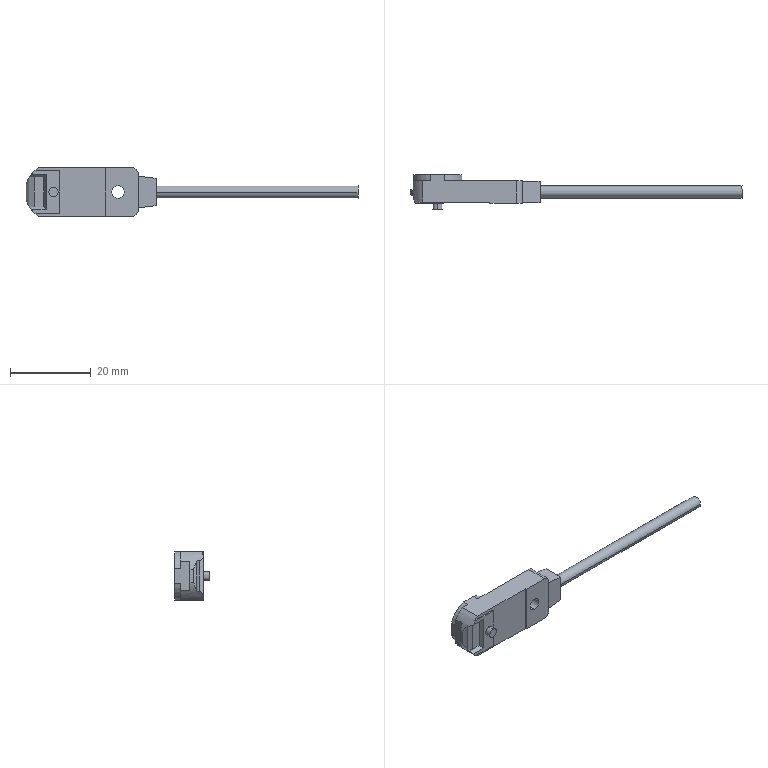Part | NX | features BREP 1 | 1 solid | 67 faces | box 82.2 x 8.6 x 12 mm | volume 2358 mm3 | plane 47 | cylinder 20 | commonest cylinder face diameters 1.5 x4 3 x4 12.5 x4 2.3 x2 3.1 x2 6 x2